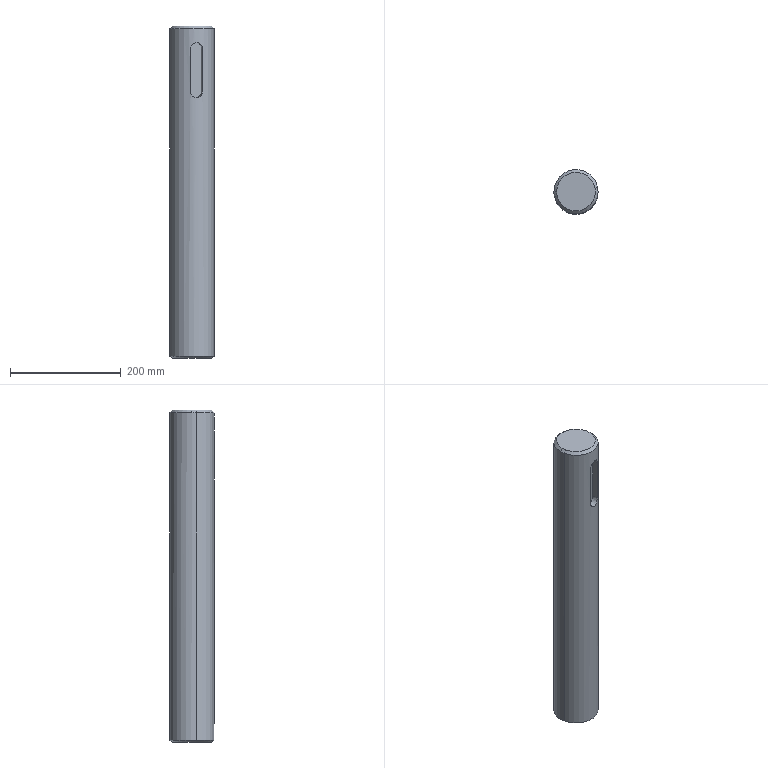Part | SolidWorks | features BaseBody 1 | 1 solid | 14 faces | box 80 x 80 x 600 mm | volume 2989143 mm3 | cone 5 | plane 5 | cylinder 4 | commonest cylinder face diameters 22 x2 80 x2
STEP:
#1=CARTESIAN_POINT('',(-722.822,509.537,864.107));
#2=VERTEX_POINT('',#1);
#3=CARTESIAN_POINT('',(-727.71,508.483,869.107));
#4=VERTEX_POINT('',#3);
#5=CARTESIAN_POINT('',(-722.822,509.537,864.107));
#6=DIRECTION('',(-0.6912,-0.1491,0.7071));
#7=VECTOR('',#6,1000.);
#8=LINE('',#5,#7);
#9=EDGE_CURVE('',#2,#4,#8,.T.);
#10=ORIENTED_EDGE('',*,*,#9,.T.);
#11=CARTESIAN_POINT('',(-796.136,493.724,869.107));
#12=VERTEX_POINT('',#11);
#13=CARTESIAN_POINT('',(-761.923,501.103,869.107));
#14=DIRECTION('',(0.,0.,1.));
#15=DIRECTION('',(1.,0.,0.));
#16=AXIS2_PLACEMENT_3D('',#13,#14,#15);
#17=CIRCLE('',#16,35.);
#18=EDGE_CURVE('',#12,#4,#17,.T.);
#19=ORIENTED_EDGE('',*,*,#18,.F.);
#20=CARTESIAN_POINT('',(-801.024,492.67,864.107));
#21=VERTEX_POINT('',#20);
#22=CARTESIAN_POINT('',(-796.136,493.724,869.107));
#23=DIRECTION('',(-0.6912,-0.1491,-0.7071));
#24=VECTOR('',#23,1000.);
#25=LINE('',#22,#24);
#26=EDGE_CURVE('',#12,#21,#25,.T.);
#27=ORIENTED_EDGE('',*,*,#26,.T.);
#28=CARTESIAN_POINT('',(-761.923,501.103,864.107));
#29=DIRECTION('',(0.,0.,-1.));
#30=DIRECTION('',(1.,0.,0.));
#31=AXIS2_PLACEMENT_3D('',#28,#29,#30);
#32=CIRCLE('',#31,40.);
#33=EDGE_CURVE('',#2,#21,#32,.T.);
#34=ORIENTED_EDGE('',*,*,#33,.F.);
#35=EDGE_LOOP('',(#10,#19,#27,#34));
#36=FACE_OUTER_BOUND('',#35,.T.);
#37=CARTESIAN_POINT('',(-761.923,501.103,864.107));
#38=DIRECTION('',(0.,0.,-1.));
#39=DIRECTION('',(-1.,0.,0.));
#40=AXIS2_PLACEMENT_3D('',#37,#38,#39);
#41=CONICAL_SURFACE('',#40,40.,0.7854);
#42=ADVANCED_FACE('',(#36),#41,.T.);
#43=CARTESIAN_POINT('',(-796.923,501.103,869.107));
#44=VERTEX_POINT('',#43);
#45=CARTESIAN_POINT('',(-801.923,501.103,864.107));
#46=VERTEX_POINT('',#45);
#47=CARTESIAN_POINT('',(-801.923,501.103,864.107));
#48=DIRECTION('',(-0.7071,0.,-0.7071));
#49=VECTOR('',#48,1000.);
#50=LINE('',#47,#49);
#51=EDGE_CURVE('',#44,#46,#50,.T.);
#52=ORIENTED_EDGE('',*,*,#51,.F.);
#53=CARTESIAN_POINT('',(-761.923,501.103,869.107));
#54=DIRECTION('',(0.,0.,1.));
#55=DIRECTION('',(1.,0.,0.));
#56=AXIS2_PLACEMENT_3D('',#53,#54,#55);
#57=CIRCLE('',#56,35.);
#58=EDGE_CURVE('',#4,#44,#57,.T.);
#59=ORIENTED_EDGE('',*,*,#58,.F.);
#60=ORIENTED_EDGE('',*,*,#9,.F.);
#61=CARTESIAN_POINT('',(-761.923,501.103,864.107));
#62=DIRECTION('',(0.,0.,-1.));
#63=DIRECTION('',(1.,0.,0.));
#64=AXIS2_PLACEMENT_3D('',#61,#62,#63);
#65=CIRCLE('',#64,40.);
#66=EDGE_CURVE('',#46,#2,#65,.T.);
#67=ORIENTED_EDGE('',*,*,#66,.F.);
#68=EDGE_LOOP('',(#52,#59,#60,#67));
#69=FACE_OUTER_BOUND('',#68,.T.);
#70=CARTESIAN_POINT('',(-761.923,501.103,864.107));
#71=DIRECTION('',(0.,0.,-1.));
#72=DIRECTION('',(-1.,0.,0.));
#73=AXIS2_PLACEMENT_3D('',#70,#71,#72);
#74=CONICAL_SURFACE('',#73,40.,0.7854);
#75=ADVANCED_FACE('',(#69),#74,.T.);
#76=CARTESIAN_POINT('',(-766.562,470.436,750.107));
#77=VERTEX_POINT('',#76);
#78=CARTESIAN_POINT('',(-745.056,475.074,750.107));
#79=VERTEX_POINT('',#78);
#80=CARTESIAN_POINT('',(-755.809,472.755,750.107));
#81=DIRECTION('',(0.2108,-0.9775,0.));
#82=DIRECTION('',(-0.9775,-0.2108,0.));
#83=AXIS2_PLACEMENT_3D('',#80,#81,#82);
#84=CIRCLE('',#83,11.);
#85=EDGE_CURVE('',#77,#79,#84,.T.);
#86=ORIENTED_EDGE('',*,*,#85,.F.);
#87=CARTESIAN_POINT('',(-764.567,461.191,750.107));
#88=VERTEX_POINT('',#87);
#89=CARTESIAN_POINT('',(-766.562,470.436,750.107));
#90=DIRECTION('',(-0.2108,0.9775,0.));
#91=VECTOR('',#90,1000.);
#92=LINE('',#89,#91);
#93=EDGE_CURVE('',#88,#77,#92,.T.);
#94=ORIENTED_EDGE('',*,*,#93,.F.);
#95=CARTESIAN_POINT('',(-743.062,465.829,750.107));
#96=VERTEX_POINT('',#95);
#97=CARTESIAN_POINT('',(-743.062,465.829,750.107));
#98=CARTESIAN_POINT('',(-743.062,465.829,749.383));
#99=CARTESIAN_POINT('',(-743.127,465.794,748.664));
#100=CARTESIAN_POINT('',(-743.322,465.691,747.6));
#101=CARTESIAN_POINT('',(-743.403,465.649,747.25));
#102=CARTESIAN_POINT('',(-743.548,465.574,746.733));
#103=CARTESIAN_POINT('',(-743.626,465.533,746.476));
#104=CARTESIAN_POINT('',(-743.713,465.488,746.221));
#105=CARTESIAN_POINT('',(-743.774,465.458,746.053));
#106=CARTESIAN_POINT('',(-743.805,465.442,745.967));
#107=CARTESIAN_POINT('',(-744.091,465.297,745.223));
#108=CARTESIAN_POINT('',(-744.403,465.142,744.591));
#109=CARTESIAN_POINT('',(-744.959,464.878,743.694));
#110=CARTESIAN_POINT('',(-745.158,464.786,743.406));
#111=CARTESIAN_POINT('',(-745.475,464.641,742.991));
#112=CARTESIAN_POINT('',(-745.585,464.592,742.855));
#113=CARTESIAN_POINT('',(-745.81,464.492,742.589));
#114=CARTESIAN_POINT('',(-745.926,464.441,742.458));
#115=CARTESIAN_POINT('',(-746.519,464.184,741.824));
#116=CARTESIAN_POINT('',(-747.036,463.972,741.371));
#117=CARTESIAN_POINT('',(-747.884,463.647,740.769));
#118=CARTESIAN_POINT('',(-748.175,463.539,740.584));
#119=CARTESIAN_POINT('',(-748.775,463.324,740.245));
#120=CARTESIAN_POINT('',(-749.082,463.219,740.092));
#121=CARTESIAN_POINT('',(-749.721,463.008,739.813));
#122=CARTESIAN_POINT('',(-750.046,462.906,739.691));
#123=CARTESIAN_POINT('',(-750.708,462.706,739.481));
#124=CARTESIAN_POINT('',(-751.043,462.61,739.393));
#125=CARTESIAN_POINT('',(-751.733,462.421,739.25));
#126=CARTESIAN_POINT('',(-752.08,462.331,739.196));
#127=CARTESIAN_POINT('',(-752.781,462.16,739.125));
#128=CARTESIAN_POINT('',(-753.136,462.079,739.107));
#129=CARTESIAN_POINT('',(-754.198,461.85,739.107));
#130=CARTESIAN_POINT('',(-754.903,461.718,739.178));
#131=CARTESIAN_POINT('',(-755.957,461.549,739.39));
#132=CARTESIAN_POINT('',(-756.304,461.498,739.478));
#133=CARTESIAN_POINT('',(-756.819,461.43,739.636));
#134=CARTESIAN_POINT('',(-756.99,461.408,739.692));
#135=CARTESIAN_POINT('',(-757.329,461.368,739.815));
#136=CARTESIAN_POINT('',(-757.499,461.348,739.881));
#137=CARTESIAN_POINT('',(-758.328,461.26,740.225));
#138=CARTESIAN_POINT('',(-758.96,461.208,740.562));
#139=CARTESIAN_POINT('',(-760.171,461.137,741.363));
#140=CARTESIAN_POINT('',(-760.734,461.118,741.819));
#141=CARTESIAN_POINT('',(-761.512,461.104,742.581));
#142=CARTESIAN_POINT('',(-761.757,461.103,742.846));
#143=CARTESIAN_POINT('',(-762.105,461.103,743.26));
#144=CARTESIAN_POINT('',(-762.218,461.104,743.401));
#145=CARTESIAN_POINT('',(-762.436,461.106,743.687));
#146=CARTESIAN_POINT('',(-762.541,461.108,743.832));
#147=CARTESIAN_POINT('',(-762.851,461.113,744.282));
#148=CARTESIAN_POINT('',(-763.041,461.118,744.59));
#149=CARTESIAN_POINT('',(-763.303,461.127,745.063));
#150=CARTESIAN_POINT('',(-763.386,461.13,745.223));
#151=CARTESIAN_POINT('',(-763.545,461.136,745.547));
#152=CARTESIAN_POINT('',(-763.62,461.139,745.709));
#153=CARTESIAN_POINT('',(-763.836,461.149,746.211));
#154=CARTESIAN_POINT('',(-763.962,461.155,746.551));
#155=CARTESIAN_POINT('',(-764.125,461.164,747.068));
#156=CARTESIAN_POINT('',(-764.175,461.167,747.241));
#157=CARTESIAN_POINT('',(-764.267,461.172,747.591));
#158=CARTESIAN_POINT('',(-764.308,461.174,747.765));
#159=CARTESIAN_POINT('',(-764.493,461.186,748.658));
#160=CARTESIAN_POINT('',(-764.567,461.191,749.379));
#161=CARTESIAN_POINT('',(-764.567,461.191,750.107));
#162=B_SPLINE_CURVE_WITH_KNOTS('',3,(#97,#98,#99,#100,#101,#102,#103,#104,#105,#106,#107,#108,#109,#110,#111,#112,#113,#114,#115,#116,#117,#118,#119,#120,#121,#122,#123,#124,#125,#126,#127,#128,#129,#130,#131,#132,#133,#134,#135,#136,#137,#138,#139,#140,#141,#142,#143,#144,#145,#146,#147,#148,#149,#150,#151,#152,#153,#154,#155,#156,#157,#158,#159,#160,#161),.UNSPECIFIED.,.F.,.F.,(4,2,2,1,2,2,2,2,2,2,2,2,2,2,2,2,2,2,2,2,2,2,2,2,2,2,2,2,2,2,2,2,4),(0.,0.0625,0.09375,0.1094,0.1172,0.125,0.1875,0.2188,0.2344,0.25,0.3125,0.3438,0.375,0.4063,0.4375,0.4688,0.5,0.5625,0.5938,0.6094,0.625,0.6875,0.75,0.7813,0.7969,0.8125,0.8438,0.8594,0.875,0.9062,0.9219,0.9375,1.),.UNSPECIFIED.);
#163=EDGE_CURVE('',#96,#88,#162,.T.);
#164=ORIENTED_EDGE('',*,*,#163,.F.);
#165=CARTESIAN_POINT('',(-743.062,465.829,750.107));
#166=DIRECTION('',(0.2108,-0.9775,0.));
#167=VECTOR('',#166,1000.);
#168=LINE('',#165,#167);
#169=EDGE_CURVE('',#79,#96,#168,.T.);
#170=ORIENTED_EDGE('',*,*,#169,.F.);
#171=EDGE_LOOP('',(#86,#94,#164,#170));
#172=FACE_OUTER_BOUND('',#171,.T.);
#173=CARTESIAN_POINT('',(-753.49,462.002,750.107));
#174=DIRECTION('',(-0.2108,0.9775,0.));
#175=DIRECTION('',(-0.9775,-0.2108,0.));
#176=AXIS2_PLACEMENT_3D('',#173,#174,#175);
#177=CYLINDRICAL_SURFACE('',#176,11.);
#178=ADVANCED_FACE('',(#172),#177,.F.);
#179=CARTESIAN_POINT('',(-743.062,465.829,828.107));
#180=VERTEX_POINT('',#179);
#181=CARTESIAN_POINT('',(-745.056,475.074,828.107));
#182=VERTEX_POINT('',#181);
#183=CARTESIAN_POINT('',(-742.737,464.322,828.107));
#184=DIRECTION('',(-0.2108,0.9775,0.));
#185=VECTOR('',#184,1000.);
#186=LINE('',#183,#185);
#187=EDGE_CURVE('',#180,#182,#186,.T.);
#188=ORIENTED_EDGE('',*,*,#187,.F.);
#189=CARTESIAN_POINT('',(-764.567,461.191,828.107));
#190=VERTEX_POINT('',#189);
#191=CARTESIAN_POINT('',(-764.567,461.191,828.107));
#192=CARTESIAN_POINT('',(-764.567,461.191,828.831));
#193=CARTESIAN_POINT('',(-764.494,461.186,829.55));
#194=CARTESIAN_POINT('',(-764.274,461.172,830.614));
#195=CARTESIAN_POINT('',(-764.183,461.167,830.963));
#196=CARTESIAN_POINT('',(-764.02,461.158,831.481));
#197=CARTESIAN_POINT('',(-763.932,461.154,831.738));
#198=CARTESIAN_POINT('',(-763.834,461.149,831.992));
#199=CARTESIAN_POINT('',(-763.766,461.146,832.161));
#200=CARTESIAN_POINT('',(-763.731,461.144,832.246));
#201=CARTESIAN_POINT('',(-763.411,461.13,832.991));
#202=CARTESIAN_POINT('',(-763.063,461.117,833.622));
#203=CARTESIAN_POINT('',(-762.447,461.106,834.519));
#204=CARTESIAN_POINT('',(-762.228,461.104,834.807));
#205=CARTESIAN_POINT('',(-761.879,461.103,835.223));
#206=CARTESIAN_POINT('',(-761.759,461.103,835.358));
#207=CARTESIAN_POINT('',(-761.513,461.105,835.625));
#208=CARTESIAN_POINT('',(-761.385,461.107,835.756));
#209=CARTESIAN_POINT('',(-760.739,461.117,836.39));
#210=CARTESIAN_POINT('',(-760.181,461.137,836.842));
#211=CARTESIAN_POINT('',(-759.274,461.19,837.444));
#212=CARTESIAN_POINT('',(-758.964,461.211,837.629));
#213=CARTESIAN_POINT('',(-758.33,461.264,837.968));
#214=CARTESIAN_POINT('',(-758.007,461.294,838.121));
#215=CARTESIAN_POINT('',(-757.338,461.365,838.4));
#216=CARTESIAN_POINT('',(-756.999,461.406,838.522));
#217=CARTESIAN_POINT('',(-756.314,461.497,838.733));
#218=CARTESIAN_POINT('',(-755.969,461.547,838.82));
#219=CARTESIAN_POINT('',(-755.263,461.66,838.964));
#220=CARTESIAN_POINT('',(-754.909,461.721,839.017));
#221=CARTESIAN_POINT('',(-754.2,461.854,839.089));
#222=CARTESIAN_POINT('',(-753.843,461.926,839.107));
#223=CARTESIAN_POINT('',(-752.782,462.155,839.107));
#224=CARTESIAN_POINT('',(-752.084,462.326,839.036));
#225=CARTESIAN_POINT('',(-751.055,462.606,838.823));
#226=CARTESIAN_POINT('',(-750.717,462.703,838.735));
#227=CARTESIAN_POINT('',(-750.22,462.853,838.578));
#228=CARTESIAN_POINT('',(-750.056,462.904,838.521));
#229=CARTESIAN_POINT('',(-749.73,463.006,838.399));
#230=CARTESIAN_POINT('',(-749.567,463.059,838.333));
#231=CARTESIAN_POINT('',(-748.775,463.32,837.988));
#232=CARTESIAN_POINT('',(-748.178,463.534,837.652));
#233=CARTESIAN_POINT('',(-747.046,463.968,836.85));
#234=CARTESIAN_POINT('',(-746.524,464.182,836.394));
#235=CARTESIAN_POINT('',(-745.811,464.491,835.632));
#236=CARTESIAN_POINT('',(-745.586,464.591,835.367));
#237=CARTESIAN_POINT('',(-745.269,464.735,834.953));
#238=CARTESIAN_POINT('',(-745.167,464.782,834.813));
#239=CARTESIAN_POINT('',(-744.969,464.874,834.526));
#240=CARTESIAN_POINT('',(-744.874,464.919,834.381));
#241=CARTESIAN_POINT('',(-744.594,465.051,833.931));
#242=CARTESIAN_POINT('',(-744.423,465.134,833.624));
#243=CARTESIAN_POINT('',(-744.188,465.25,833.15));
#244=CARTESIAN_POINT('',(-744.113,465.287,832.99));
#245=CARTESIAN_POINT('',(-743.971,465.358,832.666));
#246=CARTESIAN_POINT('',(-743.904,465.391,832.504));
#247=CARTESIAN_POINT('',(-743.711,465.489,832.002));
#248=CARTESIAN_POINT('',(-743.599,465.547,831.662));
#249=CARTESIAN_POINT('',(-743.454,465.622,831.145));
#250=CARTESIAN_POINT('',(-743.409,465.646,830.972));
#251=CARTESIAN_POINT('',(-743.328,465.688,830.622));
#252=CARTESIAN_POINT('',(-743.292,465.707,830.448));
#253=CARTESIAN_POINT('',(-743.127,465.794,829.555));
#254=CARTESIAN_POINT('',(-743.062,465.829,828.834));
#255=CARTESIAN_POINT('',(-743.062,465.829,828.107));
#256=B_SPLINE_CURVE_WITH_KNOTS('',3,(#191,#192,#193,#194,#195,#196,#197,#198,#199,#200,#201,#202,#203,#204,#205,#206,#207,#208,#209,#210,#211,#212,#213,#214,#215,#216,#217,#218,#219,#220,#221,#222,#223,#224,#225,#226,#227,#228,#229,#230,#231,#232,#233,#234,#235,#236,#237,#238,#239,#240,#241,#242,#243,#244,#245,#246,#247,#248,#249,#250,#251,#252,#253,#254,#255),.UNSPECIFIED.,.F.,.F.,(4,2,2,1,2,2,2,2,2,2,2,2,2,2,2,2,2,2,2,2,2,2,2,2,2,2,2,2,2,2,2,2,4),(0.,0.0625,0.09375,0.1094,0.1172,0.125,0.1875,0.2187,0.2344,0.25,0.3125,0.3437,0.375,0.4062,0.4375,0.4687,0.5,0.5625,0.5937,0.6094,0.625,0.6875,0.75,0.7813,0.7969,0.8125,0.8438,0.8594,0.875,0.9063,0.9219,0.9375,1.),.UNSPECIFIED.);
#257=EDGE_CURVE('',#190,#180,#256,.T.);
#258=ORIENTED_EDGE('',*,*,#257,.F.);
#259=CARTESIAN_POINT('',(-766.562,470.436,828.107));
#260=VERTEX_POINT('',#259);
#261=CARTESIAN_POINT('',(-764.242,459.683,828.107));
#262=DIRECTION('',(0.2108,-0.9775,0.));
#263=VECTOR('',#262,1000.);
#264=LINE('',#261,#263);
#265=EDGE_CURVE('',#260,#190,#264,.T.);
#266=ORIENTED_EDGE('',*,*,#265,.F.);
#267=CARTESIAN_POINT('',(-755.809,472.755,828.107));
#268=DIRECTION('',(0.2108,-0.9775,0.));
#269=DIRECTION('',(-0.9775,-0.2108,0.));
#270=AXIS2_PLACEMENT_3D('',#267,#268,#269);
#271=CIRCLE('',#270,11.);
#272=EDGE_CURVE('',#182,#260,#271,.T.);
#273=ORIENTED_EDGE('',*,*,#272,.F.);
#274=EDGE_LOOP('',(#188,#258,#266,#273));
#275=FACE_OUTER_BOUND('',#274,.T.);
#276=CARTESIAN_POINT('',(-753.49,462.002,828.107));
#277=DIRECTION('',(0.2108,-0.9775,0.));
#278=DIRECTION('',(0.9775,0.2108,0.));
#279=AXIS2_PLACEMENT_3D('',#276,#277,#278);
#280=CYLINDRICAL_SURFACE('',#279,11.);
#281=ADVANCED_FACE('',(#275),#280,.F.);
#282=CARTESIAN_POINT('',(-796.136,493.724,269.107));
#283=VERTEX_POINT('',#282);
#284=CARTESIAN_POINT('',(-801.024,492.67,271.993));
#285=VERTEX_POINT('',#284);
#286=CARTESIAN_POINT('',(-801.024,492.67,271.993));
#287=DIRECTION('',(-0.8466,-0.1826,0.5));
#288=VECTOR('',#287,1000.);
#289=LINE('',#286,#288);
#290=EDGE_CURVE('',#283,#285,#289,.T.);
#291=ORIENTED_EDGE('',*,*,#290,.T.);
#292=CARTESIAN_POINT('',(-722.822,509.537,271.993));
#293=VERTEX_POINT('',#292);
#294=CARTESIAN_POINT('',(-761.923,501.103,271.993));
#295=DIRECTION('',(0.,0.,-1.));
#296=DIRECTION('',(0.9775,0.2108,0.));
#297=AXIS2_PLACEMENT_3D('',#294,#295,#296);
#298=CIRCLE('',#297,40.);
#299=EDGE_CURVE('',#285,#293,#298,.T.);
#300=ORIENTED_EDGE('',*,*,#299,.T.);
#301=CARTESIAN_POINT('',(-727.71,508.483,269.107));
#302=VERTEX_POINT('',#301);
#303=CARTESIAN_POINT('',(-722.822,509.537,271.993));
#304=DIRECTION('',(0.8466,0.1826,0.5));
#305=VECTOR('',#304,1000.);
#306=LINE('',#303,#305);
#307=EDGE_CURVE('',#302,#293,#306,.T.);
#308=ORIENTED_EDGE('',*,*,#307,.F.);
#309=CARTESIAN_POINT('',(-761.923,501.103,269.107));
#310=DIRECTION('',(0.,0.,1.));
#311=DIRECTION('',(0.9775,0.2108,0.));
#312=AXIS2_PLACEMENT_3D('',#309,#310,#311);
#313=CIRCLE('',#312,35.);
#314=EDGE_CURVE('',#302,#283,#313,.T.);
#315=ORIENTED_EDGE('',*,*,#314,.T.);
#316=EDGE_LOOP('',(#291,#300,#308,#315));
#317=FACE_OUTER_BOUND('',#316,.T.);
#318=CARTESIAN_POINT('',(-761.923,501.103,271.993));
#319=DIRECTION('',(0.,0.,1.));
#320=DIRECTION('',(-0.9775,-0.2108,0.));
#321=AXIS2_PLACEMENT_3D('',#318,#319,#320);
#322=CONICAL_SURFACE('',#321,40.,1.047);
#323=ADVANCED_FACE('',(#317),#322,.T.);
#324=ORIENTED_EDGE('',*,*,#272,.T.);
#325=CARTESIAN_POINT('',(-766.562,470.436,739.107));
#326=DIRECTION('',(0.,0.,1.));
#327=VECTOR('',#326,1000.);
#328=LINE('',#325,#327);
#329=EDGE_CURVE('',#77,#260,#328,.T.);
#330=ORIENTED_EDGE('',*,*,#329,.F.);
#331=ORIENTED_EDGE('',*,*,#85,.T.);
#332=CARTESIAN_POINT('',(-745.056,475.074,739.107));
#333=DIRECTION('',(0.,0.,1.));
#334=VECTOR('',#333,1000.);
#335=LINE('',#332,#334);
#336=EDGE_CURVE('',#79,#182,#335,.T.);
#337=ORIENTED_EDGE('',*,*,#336,.T.);
#338=EDGE_LOOP('',(#324,#330,#331,#337));
#339=FACE_OUTER_BOUND('',#338,.T.);
#340=CARTESIAN_POINT('',(-760.696,471.701,739.107));
#341=DIRECTION('',(-0.2108,0.9775,0.));
#342=DIRECTION('',(0.,0.,1.));
#343=AXIS2_PLACEMENT_3D('',#340,#341,#342);
#344=PLANE('',#343);
#345=ADVANCED_FACE('',(#339),#344,.F.);
#346=ORIENTED_EDGE('',*,*,#329,.T.);
#347=ORIENTED_EDGE('',*,*,#265,.T.);
#348=CARTESIAN_POINT('',(-764.567,461.191,839.107));
#349=DIRECTION('',(0.,0.,-1.));
#350=VECTOR('',#349,1000.);
#351=LINE('',#348,#350);
#352=EDGE_CURVE('',#190,#88,#351,.T.);
#353=ORIENTED_EDGE('',*,*,#352,.T.);
#354=ORIENTED_EDGE('',*,*,#93,.T.);
#355=EDGE_LOOP('',(#346,#347,#353,#354));
#356=FACE_OUTER_BOUND('',#355,.T.);
#357=CARTESIAN_POINT('',(-764.242,459.683,739.107));
#358=DIRECTION('',(-0.9775,-0.2108,0.));
#359=DIRECTION('',(-0.2108,0.9775,0.));
#360=AXIS2_PLACEMENT_3D('',#357,#358,#359);
#361=PLANE('',#360);
#362=ADVANCED_FACE('',(#356),#361,.F.);
#363=CARTESIAN_POINT('',(-743.062,465.829,739.107));
#364=DIRECTION('',(0.,0.,1.));
#365=VECTOR('',#364,1000.);
#366=LINE('',#363,#365);
#367=EDGE_CURVE('',#96,#180,#366,.T.);
#368=ORIENTED_EDGE('',*,*,#367,.T.);
#369=ORIENTED_EDGE('',*,*,#187,.T.);
#370=ORIENTED_EDGE('',*,*,#336,.F.);
#371=ORIENTED_EDGE('',*,*,#169,.T.);
#372=EDGE_LOOP('',(#368,#369,#370,#371));
#373=FACE_OUTER_BOUND('',#372,.T.);
#374=CARTESIAN_POINT('',(-742.737,464.322,739.107));
#375=DIRECTION('',(0.9775,0.2108,0.));
#376=DIRECTION('',(0.,0.,-1.));
#377=AXIS2_PLACEMENT_3D('',#374,#375,#376);
#378=PLANE('',#377);
#379=ADVANCED_FACE('',(#373),#378,.F.);
#380=ORIENTED_EDGE('',*,*,#314,.F.);
#381=CARTESIAN_POINT('',(-761.923,501.103,269.107));
#382=DIRECTION('',(0.,0.,1.));
#383=DIRECTION('',(0.9775,0.2108,0.));
#384=AXIS2_PLACEMENT_3D('',#381,#382,#383);
#385=CIRCLE('',#384,35.);
#386=EDGE_CURVE('',#283,#302,#385,.T.);
#387=ORIENTED_EDGE('',*,*,#386,.F.);
#388=EDGE_LOOP('',(#380,#387));
#389=FACE_OUTER_BOUND('',#388,.T.);
#390=CARTESIAN_POINT('',(-761.923,501.103,269.107));
#391=DIRECTION('',(0.,0.,1.));
#392=DIRECTION('',(1.,0.,0.));
#393=AXIS2_PLACEMENT_3D('',#390,#391,#392);
#394=PLANE('',#393);
#395=ADVANCED_FACE('',(#389),#394,.F.);
#396=ORIENTED_EDGE('',*,*,#58,.T.);
#397=CARTESIAN_POINT('',(-761.923,501.103,869.107));
#398=DIRECTION('',(0.,0.,1.));
#399=DIRECTION('',(1.,0.,0.));
#400=AXIS2_PLACEMENT_3D('',#397,#398,#399);
#401=CIRCLE('',#400,35.);
#402=EDGE_CURVE('',#44,#12,#401,.T.);
#403=ORIENTED_EDGE('',*,*,#402,.T.);
#404=ORIENTED_EDGE('',*,*,#18,.T.);
#405=EDGE_LOOP('',(#396,#403,#404));
#406=FACE_OUTER_BOUND('',#405,.T.);
#407=CARTESIAN_POINT('',(-761.923,501.103,869.107));
#408=DIRECTION('',(0.,0.,1.));
#409=DIRECTION('',(1.,0.,0.));
#410=AXIS2_PLACEMENT_3D('',#407,#408,#409);
#411=PLANE('',#410);
#412=ADVANCED_FACE('',(#406),#411,.T.);
#413=CARTESIAN_POINT('',(-801.024,492.67,869.107));
#414=DIRECTION('',(0.,0.,-1.));
#415=VECTOR('',#414,1000.);
#416=LINE('',#413,#415);
#417=EDGE_CURVE('',#21,#285,#416,.T.);
#418=ORIENTED_EDGE('',*,*,#417,.F.);
#419=CARTESIAN_POINT('',(-761.923,501.103,864.107));
#420=DIRECTION('',(0.,0.,-1.));
#421=DIRECTION('',(1.,0.,0.));
#422=AXIS2_PLACEMENT_3D('',#419,#420,#421);
#423=CIRCLE('',#422,40.);
#424=EDGE_CURVE('',#21,#46,#423,.T.);
#425=ORIENTED_EDGE('',*,*,#424,.T.);
#426=ORIENTED_EDGE('',*,*,#66,.T.);
#427=CARTESIAN_POINT('',(-722.822,509.537,869.107));
#428=DIRECTION('',(0.,0.,-1.));
#429=VECTOR('',#428,1000.);
#430=LINE('',#427,#429);
#431=EDGE_CURVE('',#2,#293,#430,.T.);
#432=ORIENTED_EDGE('',*,*,#431,.T.);
#433=ORIENTED_EDGE('',*,*,#299,.F.);
#434=EDGE_LOOP('',(#418,#425,#426,#432,#433));
#435=FACE_OUTER_BOUND('',#434,.T.);
#436=CARTESIAN_POINT('',(-761.923,501.103,869.107));
#437=DIRECTION('',(0.,0.,-1.));
#438=DIRECTION('',(0.9775,0.2108,0.));
#439=AXIS2_PLACEMENT_3D('',#436,#437,#438);
#440=CYLINDRICAL_SURFACE('',#439,40.);
#441=ADVANCED_FACE('',(#435),#440,.T.);
#442=ORIENTED_EDGE('',*,*,#257,.T.);
#443=ORIENTED_EDGE('',*,*,#367,.F.);
#444=ORIENTED_EDGE('',*,*,#163,.T.);
#445=ORIENTED_EDGE('',*,*,#352,.F.);
#446=EDGE_LOOP('',(#442,#443,#444,#445));
#447=FACE_BOUND('',#446,.T.);
#448=ORIENTED_EDGE('',*,*,#431,.F.);
#449=ORIENTED_EDGE('',*,*,#33,.T.);
#450=ORIENTED_EDGE('',*,*,#417,.T.);
#451=CARTESIAN_POINT('',(-761.923,501.103,271.993));
#452=DIRECTION('',(0.,0.,-1.));
#453=DIRECTION('',(0.9775,0.2108,0.));
#454=AXIS2_PLACEMENT_3D('',#451,#452,#453);
#455=CIRCLE('',#454,40.);
#456=EDGE_CURVE('',#293,#285,#455,.T.);
#457=ORIENTED_EDGE('',*,*,#456,.F.);
#458=EDGE_LOOP('',(#448,#449,#450,#457));
#459=FACE_OUTER_BOUND('',#458,.T.);
#460=CARTESIAN_POINT('',(-761.923,501.103,869.107));
#461=DIRECTION('',(0.,0.,-1.));
#462=DIRECTION('',(0.9775,0.2108,0.));
#463=AXIS2_PLACEMENT_3D('',#460,#461,#462);
#464=CYLINDRICAL_SURFACE('',#463,40.);
#465=ADVANCED_FACE('',(#447,#459),#464,.T.);
#466=ORIENTED_EDGE('',*,*,#386,.T.);
#467=ORIENTED_EDGE('',*,*,#307,.T.);
#468=ORIENTED_EDGE('',*,*,#456,.T.);
#469=ORIENTED_EDGE('',*,*,#290,.F.);
#470=EDGE_LOOP('',(#466,#467,#468,#469));
#471=FACE_OUTER_BOUND('',#470,.T.);
#472=CARTESIAN_POINT('',(-761.923,501.103,271.993));
#473=DIRECTION('',(0.,0.,1.));
#474=DIRECTION('',(-0.9775,-0.2108,0.));
#475=AXIS2_PLACEMENT_3D('',#472,#473,#474);
#476=CONICAL_SURFACE('',#475,40.,1.047);
#477=ADVANCED_FACE('',(#471),#476,.T.);
#478=ORIENTED_EDGE('',*,*,#402,.F.);
#479=ORIENTED_EDGE('',*,*,#51,.T.);
#480=ORIENTED_EDGE('',*,*,#424,.F.);
#481=ORIENTED_EDGE('',*,*,#26,.F.);
#482=EDGE_LOOP('',(#478,#479,#480,#481));
#483=FACE_OUTER_BOUND('',#482,.T.);
#484=CARTESIAN_POINT('',(-761.923,501.103,864.107));
#485=DIRECTION('',(0.,0.,-1.));
#486=DIRECTION('',(-1.,0.,0.));
#487=AXIS2_PLACEMENT_3D('',#484,#485,#486);
#488=CONICAL_SURFACE('',#487,40.,0.7854);
#489=ADVANCED_FACE('',(#483),#488,.T.);
#490=CLOSED_SHELL('',(#42,#75,#178,#281,#323,#345,#362,#379,#395,#412,#441,#465,#477,#489));
#491=MANIFOLD_SOLID_BREP('',#490);
#492=CARTESIAN_POINT('',(0.,0.,0.));
#493=DIRECTION('',(0.,0.,1.));
#494=DIRECTION('',(1.,0.,0.));
#495=AXIS2_PLACEMENT_3D('',#492,#493,#494);
#496=(LENGTH_UNIT()NAMED_UNIT(*)SI_UNIT(.MILLI.,.METRE.));
#497=UNCERTAINTY_MEASURE_WITH_UNIT(LENGTH_MEASURE(0.00001),#496,'','');
#498=(NAMED_UNIT(*)PLANE_ANGLE_UNIT()SI_UNIT($,.RADIAN.));
#499=(NAMED_UNIT(*)SI_UNIT($,.STERADIAN.)SOLID_ANGLE_UNIT());
#500=(GEOMETRIC_REPRESENTATION_CONTEXT(3)GLOBAL_UNCERTAINTY_ASSIGNED_CONTEXT((#497))GLOBAL_UNIT_ASSIGNED_CONTEXT((#496,#498,#499))REPRESENTATION_CONTEXT('',''));
#501=ADVANCED_BREP_SHAPE_REPRESENTATION('',(#491,#495),#500);